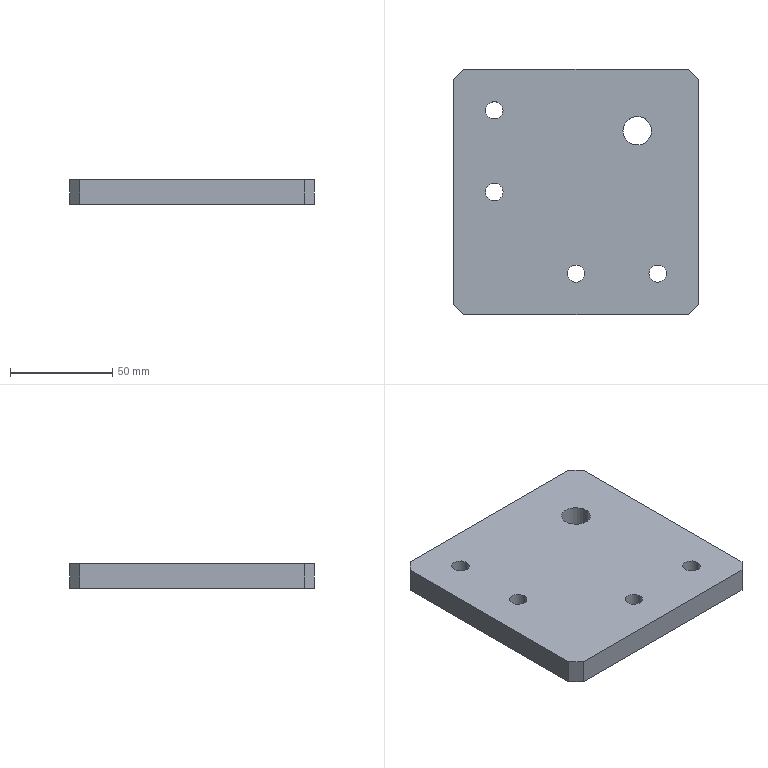Part | SolidWorks | features BaseBody 1 | 1 solid | 20 faces | box 120 x 120 x 12 mm | volume 167629 mm3 | cylinder 10 | plane 10 | commonest cylinder face diameters 8.5 x8 14 x2
STEP:
#1=CARTESIAN_POINT('',(37.,30.,-6.));
#2=VERTEX_POINT('',#1);
#3=CARTESIAN_POINT('',(23.,30.,-6.));
#4=VERTEX_POINT('',#3);
#5=CARTESIAN_POINT('',(30.,30.,-6.));
#6=DIRECTION('',(0.,0.,-1.));
#7=DIRECTION('',(-1.,0.,0.));
#8=AXIS2_PLACEMENT_3D('',#5,#6,#7);
#9=CIRCLE('',#8,7.);
#10=EDGE_CURVE('',#2,#4,#9,.T.);
#11=ORIENTED_EDGE('',*,*,#10,.T.);
#12=CARTESIAN_POINT('',(23.,30.,6.));
#13=VERTEX_POINT('',#12);
#14=CARTESIAN_POINT('',(23.,30.,6.));
#15=DIRECTION('',(0.,0.,1.));
#16=VECTOR('',#15,1000.);
#17=LINE('',#14,#16);
#18=EDGE_CURVE('',#4,#13,#17,.T.);
#19=ORIENTED_EDGE('',*,*,#18,.T.);
#20=CARTESIAN_POINT('',(37.,30.,6.));
#21=VERTEX_POINT('',#20);
#22=CARTESIAN_POINT('',(30.,30.,6.));
#23=DIRECTION('',(0.,0.,1.));
#24=DIRECTION('',(1.,0.,0.));
#25=AXIS2_PLACEMENT_3D('',#22,#23,#24);
#26=CIRCLE('',#25,7.);
#27=EDGE_CURVE('',#13,#21,#26,.T.);
#28=ORIENTED_EDGE('',*,*,#27,.T.);
#29=CARTESIAN_POINT('',(37.,30.,6.));
#30=DIRECTION('',(0.,0.,1.));
#31=VECTOR('',#30,1000.);
#32=LINE('',#29,#31);
#33=EDGE_CURVE('',#2,#21,#32,.T.);
#34=ORIENTED_EDGE('',*,*,#33,.F.);
#35=EDGE_LOOP('',(#11,#19,#28,#34));
#36=FACE_OUTER_BOUND('',#35,.T.);
#37=CARTESIAN_POINT('',(30.,30.,6.));
#38=DIRECTION('',(0.,0.,1.));
#39=DIRECTION('',(1.,0.,0.));
#40=AXIS2_PLACEMENT_3D('',#37,#38,#39);
#41=CYLINDRICAL_SURFACE('',#40,7.);
#42=ADVANCED_FACE('',(#36),#41,.F.);
#43=CARTESIAN_POINT('',(-4.25,-40.,-6.));
#44=VERTEX_POINT('',#43);
#45=CARTESIAN_POINT('',(4.25,-40.,-6.));
#46=VERTEX_POINT('',#45);
#47=CARTESIAN_POINT('',(0.,-40.,-6.));
#48=DIRECTION('',(0.,0.,1.));
#49=DIRECTION('',(1.,0.,0.));
#50=AXIS2_PLACEMENT_3D('',#47,#48,#49);
#51=CIRCLE('',#50,4.25);
#52=EDGE_CURVE('',#44,#46,#51,.T.);
#53=ORIENTED_EDGE('',*,*,#52,.F.);
#54=CARTESIAN_POINT('',(-4.25,-40.,6.));
#55=VERTEX_POINT('',#54);
#56=CARTESIAN_POINT('',(-4.25,-40.,-6.));
#57=DIRECTION('',(0.,0.,1.));
#58=VECTOR('',#57,1000.);
#59=LINE('',#56,#58);
#60=EDGE_CURVE('',#44,#55,#59,.T.);
#61=ORIENTED_EDGE('',*,*,#60,.T.);
#62=CARTESIAN_POINT('',(4.25,-40.,6.));
#63=VERTEX_POINT('',#62);
#64=CARTESIAN_POINT('',(0.,-40.,6.));
#65=DIRECTION('',(0.,0.,1.));
#66=DIRECTION('',(1.,0.,0.));
#67=AXIS2_PLACEMENT_3D('',#64,#65,#66);
#68=CIRCLE('',#67,4.25);
#69=EDGE_CURVE('',#55,#63,#68,.T.);
#70=ORIENTED_EDGE('',*,*,#69,.T.);
#71=CARTESIAN_POINT('',(4.25,-40.,-6.));
#72=DIRECTION('',(0.,0.,1.));
#73=VECTOR('',#72,1000.);
#74=LINE('',#71,#73);
#75=EDGE_CURVE('',#46,#63,#74,.T.);
#76=ORIENTED_EDGE('',*,*,#75,.F.);
#77=EDGE_LOOP('',(#53,#61,#70,#76));
#78=FACE_OUTER_BOUND('',#77,.T.);
#79=CARTESIAN_POINT('',(0.,-40.,-6.));
#80=DIRECTION('',(0.,0.,1.));
#81=DIRECTION('',(1.,0.,0.));
#82=AXIS2_PLACEMENT_3D('',#79,#80,#81);
#83=CYLINDRICAL_SURFACE('',#82,4.25);
#84=ADVANCED_FACE('',(#78),#83,.F.);
#85=CARTESIAN_POINT('',(35.75,-40.,-6.));
#86=VERTEX_POINT('',#85);
#87=CARTESIAN_POINT('',(44.25,-40.,-6.));
#88=VERTEX_POINT('',#87);
#89=CARTESIAN_POINT('',(40.,-40.,-6.));
#90=DIRECTION('',(0.,0.,1.));
#91=DIRECTION('',(1.,0.,0.));
#92=AXIS2_PLACEMENT_3D('',#89,#90,#91);
#93=CIRCLE('',#92,4.25);
#94=EDGE_CURVE('',#86,#88,#93,.T.);
#95=ORIENTED_EDGE('',*,*,#94,.F.);
#96=CARTESIAN_POINT('',(35.75,-40.,6.));
#97=VERTEX_POINT('',#96);
#98=CARTESIAN_POINT('',(35.75,-40.,-6.));
#99=DIRECTION('',(0.,0.,1.));
#100=VECTOR('',#99,1000.);
#101=LINE('',#98,#100);
#102=EDGE_CURVE('',#86,#97,#101,.T.);
#103=ORIENTED_EDGE('',*,*,#102,.T.);
#104=CARTESIAN_POINT('',(44.25,-40.,6.));
#105=VERTEX_POINT('',#104);
#106=CARTESIAN_POINT('',(40.,-40.,6.));
#107=DIRECTION('',(0.,0.,1.));
#108=DIRECTION('',(1.,0.,0.));
#109=AXIS2_PLACEMENT_3D('',#106,#107,#108);
#110=CIRCLE('',#109,4.25);
#111=EDGE_CURVE('',#97,#105,#110,.T.);
#112=ORIENTED_EDGE('',*,*,#111,.T.);
#113=CARTESIAN_POINT('',(44.25,-40.,-6.));
#114=DIRECTION('',(0.,0.,1.));
#115=VECTOR('',#114,1000.);
#116=LINE('',#113,#115);
#117=EDGE_CURVE('',#88,#105,#116,.T.);
#118=ORIENTED_EDGE('',*,*,#117,.F.);
#119=EDGE_LOOP('',(#95,#103,#112,#118));
#120=FACE_OUTER_BOUND('',#119,.T.);
#121=CARTESIAN_POINT('',(40.,-40.,-6.));
#122=DIRECTION('',(0.,0.,1.));
#123=DIRECTION('',(1.,0.,0.));
#124=AXIS2_PLACEMENT_3D('',#121,#122,#123);
#125=CYLINDRICAL_SURFACE('',#124,4.25);
#126=ADVANCED_FACE('',(#120),#125,.F.);
#127=CARTESIAN_POINT('',(-44.25,0.,-6.));
#128=VERTEX_POINT('',#127);
#129=CARTESIAN_POINT('',(-35.75,0.,-6.));
#130=VERTEX_POINT('',#129);
#131=CARTESIAN_POINT('',(-40.,0.,-6.));
#132=DIRECTION('',(0.,0.,1.));
#133=DIRECTION('',(1.,0.,0.));
#134=AXIS2_PLACEMENT_3D('',#131,#132,#133);
#135=CIRCLE('',#134,4.25);
#136=EDGE_CURVE('',#128,#130,#135,.T.);
#137=ORIENTED_EDGE('',*,*,#136,.F.);
#138=CARTESIAN_POINT('',(-44.25,0.,6.));
#139=VERTEX_POINT('',#138);
#140=CARTESIAN_POINT('',(-44.25,0.,-6.));
#141=DIRECTION('',(0.,0.,1.));
#142=VECTOR('',#141,1000.);
#143=LINE('',#140,#142);
#144=EDGE_CURVE('',#128,#139,#143,.T.);
#145=ORIENTED_EDGE('',*,*,#144,.T.);
#146=CARTESIAN_POINT('',(-35.75,0.,6.));
#147=VERTEX_POINT('',#146);
#148=CARTESIAN_POINT('',(-40.,0.,6.));
#149=DIRECTION('',(0.,0.,1.));
#150=DIRECTION('',(1.,0.,0.));
#151=AXIS2_PLACEMENT_3D('',#148,#149,#150);
#152=CIRCLE('',#151,4.25);
#153=EDGE_CURVE('',#139,#147,#152,.T.);
#154=ORIENTED_EDGE('',*,*,#153,.T.);
#155=CARTESIAN_POINT('',(-35.75,0.,-6.));
#156=DIRECTION('',(0.,0.,1.));
#157=VECTOR('',#156,1000.);
#158=LINE('',#155,#157);
#159=EDGE_CURVE('',#130,#147,#158,.T.);
#160=ORIENTED_EDGE('',*,*,#159,.F.);
#161=EDGE_LOOP('',(#137,#145,#154,#160));
#162=FACE_OUTER_BOUND('',#161,.T.);
#163=CARTESIAN_POINT('',(-40.,0.,-6.));
#164=DIRECTION('',(0.,0.,1.));
#165=DIRECTION('',(1.,0.,0.));
#166=AXIS2_PLACEMENT_3D('',#163,#164,#165);
#167=CYLINDRICAL_SURFACE('',#166,4.25);
#168=ADVANCED_FACE('',(#162),#167,.F.);
#169=CARTESIAN_POINT('',(-44.25,40.,-6.));
#170=VERTEX_POINT('',#169);
#171=CARTESIAN_POINT('',(-35.75,40.,-6.));
#172=VERTEX_POINT('',#171);
#173=CARTESIAN_POINT('',(-40.,40.,-6.));
#174=DIRECTION('',(0.,0.,1.));
#175=DIRECTION('',(1.,0.,0.));
#176=AXIS2_PLACEMENT_3D('',#173,#174,#175);
#177=CIRCLE('',#176,4.25);
#178=EDGE_CURVE('',#170,#172,#177,.T.);
#179=ORIENTED_EDGE('',*,*,#178,.F.);
#180=CARTESIAN_POINT('',(-44.25,40.,6.));
#181=VERTEX_POINT('',#180);
#182=CARTESIAN_POINT('',(-44.25,40.,-6.));
#183=DIRECTION('',(0.,0.,1.));
#184=VECTOR('',#183,1000.);
#185=LINE('',#182,#184);
#186=EDGE_CURVE('',#170,#181,#185,.T.);
#187=ORIENTED_EDGE('',*,*,#186,.T.);
#188=CARTESIAN_POINT('',(-35.75,40.,6.));
#189=VERTEX_POINT('',#188);
#190=CARTESIAN_POINT('',(-40.,40.,6.));
#191=DIRECTION('',(0.,0.,1.));
#192=DIRECTION('',(1.,0.,0.));
#193=AXIS2_PLACEMENT_3D('',#190,#191,#192);
#194=CIRCLE('',#193,4.25);
#195=EDGE_CURVE('',#181,#189,#194,.T.);
#196=ORIENTED_EDGE('',*,*,#195,.T.);
#197=CARTESIAN_POINT('',(-35.75,40.,-6.));
#198=DIRECTION('',(0.,0.,1.));
#199=VECTOR('',#198,1000.);
#200=LINE('',#197,#199);
#201=EDGE_CURVE('',#172,#189,#200,.T.);
#202=ORIENTED_EDGE('',*,*,#201,.F.);
#203=EDGE_LOOP('',(#179,#187,#196,#202));
#204=FACE_OUTER_BOUND('',#203,.T.);
#205=CARTESIAN_POINT('',(-40.,40.,-6.));
#206=DIRECTION('',(0.,0.,1.));
#207=DIRECTION('',(1.,0.,0.));
#208=AXIS2_PLACEMENT_3D('',#205,#206,#207);
#209=CYLINDRICAL_SURFACE('',#208,4.25);
#210=ADVANCED_FACE('',(#204),#209,.F.);
#211=CARTESIAN_POINT('',(-60.,55.,6.));
#212=VERTEX_POINT('',#211);
#213=CARTESIAN_POINT('',(-60.,-55.,6.));
#214=VERTEX_POINT('',#213);
#215=CARTESIAN_POINT('',(-60.,60.,6.));
#216=DIRECTION('',(0.,-1.,0.));
#217=VECTOR('',#216,1000.);
#218=LINE('',#215,#217);
#219=EDGE_CURVE('',#212,#214,#218,.T.);
#220=ORIENTED_EDGE('',*,*,#219,.F.);
#221=CARTESIAN_POINT('',(-60.,55.,-6.));
#222=VERTEX_POINT('',#221);
#223=CARTESIAN_POINT('',(-60.,55.,6.));
#224=DIRECTION('',(0.,0.,-1.));
#225=VECTOR('',#224,1000.);
#226=LINE('',#223,#225);
#227=EDGE_CURVE('',#212,#222,#226,.T.);
#228=ORIENTED_EDGE('',*,*,#227,.T.);
#229=CARTESIAN_POINT('',(-60.,-55.,-6.));
#230=VERTEX_POINT('',#229);
#231=CARTESIAN_POINT('',(-60.,60.,-6.));
#232=DIRECTION('',(0.,-1.,0.));
#233=VECTOR('',#232,1000.);
#234=LINE('',#231,#233);
#235=EDGE_CURVE('',#222,#230,#234,.T.);
#236=ORIENTED_EDGE('',*,*,#235,.T.);
#237=CARTESIAN_POINT('',(-60.,-55.,6.));
#238=DIRECTION('',(0.,0.,1.));
#239=VECTOR('',#238,1000.);
#240=LINE('',#237,#239);
#241=EDGE_CURVE('',#230,#214,#240,.T.);
#242=ORIENTED_EDGE('',*,*,#241,.T.);
#243=EDGE_LOOP('',(#220,#228,#236,#242));
#244=FACE_OUTER_BOUND('',#243,.T.);
#245=CARTESIAN_POINT('',(-60.,60.,6.));
#246=DIRECTION('',(1.,0.,0.));
#247=DIRECTION('',(0.,1.,0.));
#248=AXIS2_PLACEMENT_3D('',#245,#246,#247);
#249=PLANE('',#248);
#250=ADVANCED_FACE('',(#244),#249,.F.);
#251=CARTESIAN_POINT('',(-55.,-60.,-6.));
#252=VERTEX_POINT('',#251);
#253=CARTESIAN_POINT('',(55.,-60.,-6.));
#254=VERTEX_POINT('',#253);
#255=CARTESIAN_POINT('',(60.,-60.,-6.));
#256=DIRECTION('',(1.,0.,0.));
#257=VECTOR('',#256,1000.);
#258=LINE('',#255,#257);
#259=EDGE_CURVE('',#252,#254,#258,.T.);
#260=ORIENTED_EDGE('',*,*,#259,.T.);
#261=CARTESIAN_POINT('',(55.,-60.,6.));
#262=VERTEX_POINT('',#261);
#263=CARTESIAN_POINT('',(55.,-60.,6.));
#264=DIRECTION('',(0.,0.,1.));
#265=VECTOR('',#264,1000.);
#266=LINE('',#263,#265);
#267=EDGE_CURVE('',#254,#262,#266,.T.);
#268=ORIENTED_EDGE('',*,*,#267,.T.);
#269=CARTESIAN_POINT('',(-55.,-60.,6.));
#270=VERTEX_POINT('',#269);
#271=CARTESIAN_POINT('',(60.,-60.,6.));
#272=DIRECTION('',(1.,0.,0.));
#273=VECTOR('',#272,1000.);
#274=LINE('',#271,#273);
#275=EDGE_CURVE('',#270,#262,#274,.T.);
#276=ORIENTED_EDGE('',*,*,#275,.F.);
#277=CARTESIAN_POINT('',(-55.,-60.,6.));
#278=DIRECTION('',(0.,0.,-1.));
#279=VECTOR('',#278,1000.);
#280=LINE('',#277,#279);
#281=EDGE_CURVE('',#270,#252,#280,.T.);
#282=ORIENTED_EDGE('',*,*,#281,.T.);
#283=EDGE_LOOP('',(#260,#268,#276,#282));
#284=FACE_OUTER_BOUND('',#283,.T.);
#285=CARTESIAN_POINT('',(60.,-60.,6.));
#286=DIRECTION('',(0.,1.,0.));
#287=DIRECTION('',(-1.,0.,0.));
#288=AXIS2_PLACEMENT_3D('',#285,#286,#287);
#289=PLANE('',#288);
#290=ADVANCED_FACE('',(#284),#289,.F.);
#291=CARTESIAN_POINT('',(60.,-55.,-6.));
#292=VERTEX_POINT('',#291);
#293=CARTESIAN_POINT('',(60.,55.,-6.));
#294=VERTEX_POINT('',#293);
#295=CARTESIAN_POINT('',(60.,60.,-6.));
#296=DIRECTION('',(0.,1.,0.));
#297=VECTOR('',#296,1000.);
#298=LINE('',#295,#297);
#299=EDGE_CURVE('',#292,#294,#298,.T.);
#300=ORIENTED_EDGE('',*,*,#299,.T.);
#301=CARTESIAN_POINT('',(60.,55.,6.));
#302=VERTEX_POINT('',#301);
#303=CARTESIAN_POINT('',(60.,55.,6.));
#304=DIRECTION('',(0.,0.,1.));
#305=VECTOR('',#304,1000.);
#306=LINE('',#303,#305);
#307=EDGE_CURVE('',#294,#302,#306,.T.);
#308=ORIENTED_EDGE('',*,*,#307,.T.);
#309=CARTESIAN_POINT('',(60.,-55.,6.));
#310=VERTEX_POINT('',#309);
#311=CARTESIAN_POINT('',(60.,60.,6.));
#312=DIRECTION('',(0.,1.,0.));
#313=VECTOR('',#312,1000.);
#314=LINE('',#311,#313);
#315=EDGE_CURVE('',#310,#302,#314,.T.);
#316=ORIENTED_EDGE('',*,*,#315,.F.);
#317=CARTESIAN_POINT('',(60.,-55.,6.));
#318=DIRECTION('',(0.,0.,-1.));
#319=VECTOR('',#318,1000.);
#320=LINE('',#317,#319);
#321=EDGE_CURVE('',#310,#292,#320,.T.);
#322=ORIENTED_EDGE('',*,*,#321,.T.);
#323=EDGE_LOOP('',(#300,#308,#316,#322));
#324=FACE_OUTER_BOUND('',#323,.T.);
#325=CARTESIAN_POINT('',(60.,60.,6.));
#326=DIRECTION('',(-1.,0.,0.));
#327=DIRECTION('',(0.,-1.,0.));
#328=AXIS2_PLACEMENT_3D('',#325,#326,#327);
#329=PLANE('',#328);
#330=ADVANCED_FACE('',(#324),#329,.F.);
#331=CARTESIAN_POINT('',(55.,60.,6.));
#332=VERTEX_POINT('',#331);
#333=CARTESIAN_POINT('',(-55.,60.,6.));
#334=VERTEX_POINT('',#333);
#335=CARTESIAN_POINT('',(60.,60.,6.));
#336=DIRECTION('',(-1.,0.,0.));
#337=VECTOR('',#336,1000.);
#338=LINE('',#335,#337);
#339=EDGE_CURVE('',#332,#334,#338,.T.);
#340=ORIENTED_EDGE('',*,*,#339,.F.);
#341=CARTESIAN_POINT('',(55.,60.,-6.));
#342=VERTEX_POINT('',#341);
#343=CARTESIAN_POINT('',(55.,60.,6.));
#344=DIRECTION('',(0.,0.,-1.));
#345=VECTOR('',#344,1000.);
#346=LINE('',#343,#345);
#347=EDGE_CURVE('',#332,#342,#346,.T.);
#348=ORIENTED_EDGE('',*,*,#347,.T.);
#349=CARTESIAN_POINT('',(-55.,60.,-6.));
#350=VERTEX_POINT('',#349);
#351=CARTESIAN_POINT('',(60.,60.,-6.));
#352=DIRECTION('',(-1.,0.,0.));
#353=VECTOR('',#352,1000.);
#354=LINE('',#351,#353);
#355=EDGE_CURVE('',#342,#350,#354,.T.);
#356=ORIENTED_EDGE('',*,*,#355,.T.);
#357=CARTESIAN_POINT('',(-55.,60.,6.));
#358=DIRECTION('',(0.,0.,1.));
#359=VECTOR('',#358,1000.);
#360=LINE('',#357,#359);
#361=EDGE_CURVE('',#350,#334,#360,.T.);
#362=ORIENTED_EDGE('',*,*,#361,.T.);
#363=EDGE_LOOP('',(#340,#348,#356,#362));
#364=FACE_OUTER_BOUND('',#363,.T.);
#365=CARTESIAN_POINT('',(60.,60.,6.));
#366=DIRECTION('',(0.,-1.,0.));
#367=DIRECTION('',(1.,0.,0.));
#368=AXIS2_PLACEMENT_3D('',#365,#366,#367);
#369=PLANE('',#368);
#370=ADVANCED_FACE('',(#364),#369,.F.);
#371=CARTESIAN_POINT('',(30.,30.,6.));
#372=DIRECTION('',(0.,0.,1.));
#373=DIRECTION('',(1.,0.,0.));
#374=AXIS2_PLACEMENT_3D('',#371,#372,#373);
#375=CIRCLE('',#374,7.);
#376=EDGE_CURVE('',#21,#13,#375,.T.);
#377=ORIENTED_EDGE('',*,*,#376,.F.);
#378=ORIENTED_EDGE('',*,*,#27,.F.);
#379=EDGE_LOOP('',(#377,#378));
#380=FACE_BOUND('',#379,.T.);
#381=CARTESIAN_POINT('',(0.,-40.,6.));
#382=DIRECTION('',(0.,0.,1.));
#383=DIRECTION('',(1.,0.,0.));
#384=AXIS2_PLACEMENT_3D('',#381,#382,#383);
#385=CIRCLE('',#384,4.25);
#386=EDGE_CURVE('',#63,#55,#385,.T.);
#387=ORIENTED_EDGE('',*,*,#386,.F.);
#388=ORIENTED_EDGE('',*,*,#69,.F.);
#389=EDGE_LOOP('',(#387,#388));
#390=FACE_BOUND('',#389,.T.);
#391=CARTESIAN_POINT('',(40.,-40.,6.));
#392=DIRECTION('',(0.,0.,1.));
#393=DIRECTION('',(1.,0.,0.));
#394=AXIS2_PLACEMENT_3D('',#391,#392,#393);
#395=CIRCLE('',#394,4.25);
#396=EDGE_CURVE('',#105,#97,#395,.T.);
#397=ORIENTED_EDGE('',*,*,#396,.F.);
#398=ORIENTED_EDGE('',*,*,#111,.F.);
#399=EDGE_LOOP('',(#397,#398));
#400=FACE_BOUND('',#399,.T.);
#401=CARTESIAN_POINT('',(-40.,0.,6.));
#402=DIRECTION('',(0.,0.,1.));
#403=DIRECTION('',(1.,0.,0.));
#404=AXIS2_PLACEMENT_3D('',#401,#402,#403);
#405=CIRCLE('',#404,4.25);
#406=EDGE_CURVE('',#147,#139,#405,.T.);
#407=ORIENTED_EDGE('',*,*,#406,.F.);
#408=ORIENTED_EDGE('',*,*,#153,.F.);
#409=EDGE_LOOP('',(#407,#408));
#410=FACE_BOUND('',#409,.T.);
#411=CARTESIAN_POINT('',(-40.,40.,6.));
#412=DIRECTION('',(0.,0.,1.));
#413=DIRECTION('',(1.,0.,0.));
#414=AXIS2_PLACEMENT_3D('',#411,#412,#413);
#415=CIRCLE('',#414,4.25);
#416=EDGE_CURVE('',#189,#181,#415,.T.);
#417=ORIENTED_EDGE('',*,*,#416,.F.);
#418=ORIENTED_EDGE('',*,*,#195,.F.);
#419=EDGE_LOOP('',(#417,#418));
#420=FACE_BOUND('',#419,.T.);
#421=ORIENTED_EDGE('',*,*,#315,.T.);
#422=CARTESIAN_POINT('',(55.,60.,6.));
#423=DIRECTION('',(-0.7071,0.7071,0.));
#424=VECTOR('',#423,1000.);
#425=LINE('',#422,#424);
#426=EDGE_CURVE('',#302,#332,#425,.T.);
#427=ORIENTED_EDGE('',*,*,#426,.T.);
#428=ORIENTED_EDGE('',*,*,#339,.T.);
#429=CARTESIAN_POINT('',(-60.,55.,6.));
#430=DIRECTION('',(-0.7071,-0.7071,0.));
#431=VECTOR('',#430,1000.);
#432=LINE('',#429,#431);
#433=EDGE_CURVE('',#334,#212,#432,.T.);
#434=ORIENTED_EDGE('',*,*,#433,.T.);
#435=ORIENTED_EDGE('',*,*,#219,.T.);
#436=CARTESIAN_POINT('',(-55.,-60.,6.));
#437=DIRECTION('',(0.7071,-0.7071,0.));
#438=VECTOR('',#437,1000.);
#439=LINE('',#436,#438);
#440=EDGE_CURVE('',#214,#270,#439,.T.);
#441=ORIENTED_EDGE('',*,*,#440,.T.);
#442=ORIENTED_EDGE('',*,*,#275,.T.);
#443=CARTESIAN_POINT('',(60.,-55.,6.));
#444=DIRECTION('',(0.7071,0.7071,0.));
#445=VECTOR('',#444,1000.);
#446=LINE('',#443,#445);
#447=EDGE_CURVE('',#262,#310,#446,.T.);
#448=ORIENTED_EDGE('',*,*,#447,.T.);
#449=EDGE_LOOP('',(#421,#427,#428,#434,#435,#441,#442,#448));
#450=FACE_OUTER_BOUND('',#449,.T.);
#451=CARTESIAN_POINT('',(-60.,-60.,6.));
#452=DIRECTION('',(0.,0.,-1.));
#453=DIRECTION('',(-1.,0.,0.));
#454=AXIS2_PLACEMENT_3D('',#451,#452,#453);
#455=PLANE('',#454);
#456=ADVANCED_FACE('',(#380,#390,#400,#410,#420,#450),#455,.F.);
#457=ORIENTED_EDGE('',*,*,#10,.F.);
#458=CARTESIAN_POINT('',(30.,30.,-6.));
#459=DIRECTION('',(0.,0.,-1.));
#460=DIRECTION('',(-1.,0.,0.));
#461=AXIS2_PLACEMENT_3D('',#458,#459,#460);
#462=CIRCLE('',#461,7.);
#463=EDGE_CURVE('',#4,#2,#462,.T.);
#464=ORIENTED_EDGE('',*,*,#463,.F.);
#465=EDGE_LOOP('',(#457,#464));
#466=FACE_BOUND('',#465,.T.);
#467=CARTESIAN_POINT('',(0.,-40.,-6.));
#468=DIRECTION('',(0.,0.,1.));
#469=DIRECTION('',(1.,0.,0.));
#470=AXIS2_PLACEMENT_3D('',#467,#468,#469);
#471=CIRCLE('',#470,4.25);
#472=EDGE_CURVE('',#46,#44,#471,.T.);
#473=ORIENTED_EDGE('',*,*,#472,.T.);
#474=ORIENTED_EDGE('',*,*,#52,.T.);
#475=EDGE_LOOP('',(#473,#474));
#476=FACE_BOUND('',#475,.T.);
#477=CARTESIAN_POINT('',(40.,-40.,-6.));
#478=DIRECTION('',(0.,0.,1.));
#479=DIRECTION('',(1.,0.,0.));
#480=AXIS2_PLACEMENT_3D('',#477,#478,#479);
#481=CIRCLE('',#480,4.25);
#482=EDGE_CURVE('',#88,#86,#481,.T.);
#483=ORIENTED_EDGE('',*,*,#482,.T.);
#484=ORIENTED_EDGE('',*,*,#94,.T.);
#485=EDGE_LOOP('',(#483,#484));
#486=FACE_BOUND('',#485,.T.);
#487=CARTESIAN_POINT('',(-40.,0.,-6.));
#488=DIRECTION('',(0.,0.,1.));
#489=DIRECTION('',(1.,0.,0.));
#490=AXIS2_PLACEMENT_3D('',#487,#488,#489);
#491=CIRCLE('',#490,4.25);
#492=EDGE_CURVE('',#130,#128,#491,.T.);
#493=ORIENTED_EDGE('',*,*,#492,.T.);
#494=ORIENTED_EDGE('',*,*,#136,.T.);
#495=EDGE_LOOP('',(#493,#494));
#496=FACE_BOUND('',#495,.T.);
#497=CARTESIAN_POINT('',(-40.,40.,-6.));
#498=DIRECTION('',(0.,0.,1.));
#499=DIRECTION('',(1.,0.,0.));
#500=AXIS2_PLACEMENT_3D('',#497,#498,#499);
#501=CIRCLE('',#500,4.25);
#502=EDGE_CURVE('',#172,#170,#501,.T.);
#503=ORIENTED_EDGE('',*,*,#502,.T.);
#504=ORIENTED_EDGE('',*,*,#178,.T.);
#505=EDGE_LOOP('',(#503,#504));
#506=FACE_BOUND('',#505,.T.);
#507=ORIENTED_EDGE('',*,*,#355,.F.);
#508=CARTESIAN_POINT('',(57.5,57.5,-6.));
#509=DIRECTION('',(0.7071,-0.7071,0.));
#510=VECTOR('',#509,1000.);
#511=LINE('',#508,#510);
#512=EDGE_CURVE('',#342,#294,#511,.T.);
#513=ORIENTED_EDGE('',*,*,#512,.T.);
#514=ORIENTED_EDGE('',*,*,#299,.F.);
#515=CARTESIAN_POINT('',(-2.5,-117.5,-6.));
#516=DIRECTION('',(-0.7071,-0.7071,0.));
#517=VECTOR('',#516,1000.);
#518=LINE('',#515,#517);
#519=EDGE_CURVE('',#292,#254,#518,.T.);
#520=ORIENTED_EDGE('',*,*,#519,.T.);
#521=ORIENTED_EDGE('',*,*,#259,.F.);
#522=CARTESIAN_POINT('',(-57.5,-57.5,-6.));
#523=DIRECTION('',(-0.7071,0.7071,0.));
#524=VECTOR('',#523,1000.);
#525=LINE('',#522,#524);
#526=EDGE_CURVE('',#252,#230,#525,.T.);
#527=ORIENTED_EDGE('',*,*,#526,.T.);
#528=ORIENTED_EDGE('',*,*,#235,.F.);
#529=CARTESIAN_POINT('',(-117.5,-2.5,-6.));
#530=DIRECTION('',(0.7071,0.7071,0.));
#531=VECTOR('',#530,1000.);
#532=LINE('',#529,#531);
#533=EDGE_CURVE('',#222,#350,#532,.T.);
#534=ORIENTED_EDGE('',*,*,#533,.T.);
#535=EDGE_LOOP('',(#507,#513,#514,#520,#521,#527,#528,#534));
#536=FACE_OUTER_BOUND('',#535,.T.);
#537=CARTESIAN_POINT('',(-60.,-60.,-6.));
#538=DIRECTION('',(0.,0.,-1.));
#539=DIRECTION('',(-1.,0.,0.));
#540=AXIS2_PLACEMENT_3D('',#537,#538,#539);
#541=PLANE('',#540);
#542=ADVANCED_FACE('',(#466,#476,#486,#496,#506,#536),#541,.T.);
#543=ORIENTED_EDGE('',*,*,#186,.F.);
#544=ORIENTED_EDGE('',*,*,#502,.F.);
#545=ORIENTED_EDGE('',*,*,#201,.T.);
#546=ORIENTED_EDGE('',*,*,#416,.T.);
#547=EDGE_LOOP('',(#543,#544,#545,#546));
#548=FACE_OUTER_BOUND('',#547,.T.);
#549=CARTESIAN_POINT('',(-40.,40.,-6.));
#550=DIRECTION('',(0.,0.,1.));
#551=DIRECTION('',(1.,0.,0.));
#552=AXIS2_PLACEMENT_3D('',#549,#550,#551);
#553=CYLINDRICAL_SURFACE('',#552,4.25);
#554=ADVANCED_FACE('',(#548),#553,.F.);
#555=ORIENTED_EDGE('',*,*,#144,.F.);
#556=ORIENTED_EDGE('',*,*,#492,.F.);
#557=ORIENTED_EDGE('',*,*,#159,.T.);
#558=ORIENTED_EDGE('',*,*,#406,.T.);
#559=EDGE_LOOP('',(#555,#556,#557,#558));
#560=FACE_OUTER_BOUND('',#559,.T.);
#561=CARTESIAN_POINT('',(-40.,0.,-6.));
#562=DIRECTION('',(0.,0.,1.));
#563=DIRECTION('',(1.,0.,0.));
#564=AXIS2_PLACEMENT_3D('',#561,#562,#563);
#565=CYLINDRICAL_SURFACE('',#564,4.25);
#566=ADVANCED_FACE('',(#560),#565,.F.);
#567=ORIENTED_EDGE('',*,*,#102,.F.);
#568=ORIENTED_EDGE('',*,*,#482,.F.);
#569=ORIENTED_EDGE('',*,*,#117,.T.);
#570=ORIENTED_EDGE('',*,*,#396,.T.);
#571=EDGE_LOOP('',(#567,#568,#569,#570));
#572=FACE_OUTER_BOUND('',#571,.T.);
#573=CARTESIAN_POINT('',(40.,-40.,-6.));
#574=DIRECTION('',(0.,0.,1.));
#575=DIRECTION('',(1.,0.,0.));
#576=AXIS2_PLACEMENT_3D('',#573,#574,#575);
#577=CYLINDRICAL_SURFACE('',#576,4.25);
#578=ADVANCED_FACE('',(#572),#577,.F.);
#579=ORIENTED_EDGE('',*,*,#60,.F.);
#580=ORIENTED_EDGE('',*,*,#472,.F.);
#581=ORIENTED_EDGE('',*,*,#75,.T.);
#582=ORIENTED_EDGE('',*,*,#386,.T.);
#583=EDGE_LOOP('',(#579,#580,#581,#582));
#584=FACE_OUTER_BOUND('',#583,.T.);
#585=CARTESIAN_POINT('',(0.,-40.,-6.));
#586=DIRECTION('',(0.,0.,1.));
#587=DIRECTION('',(1.,0.,0.));
#588=AXIS2_PLACEMENT_3D('',#585,#586,#587);
#589=CYLINDRICAL_SURFACE('',#588,4.25);
#590=ADVANCED_FACE('',(#584),#589,.F.);
#591=ORIENTED_EDGE('',*,*,#18,.F.);
#592=ORIENTED_EDGE('',*,*,#463,.T.);
#593=ORIENTED_EDGE('',*,*,#33,.T.);
#594=ORIENTED_EDGE('',*,*,#376,.T.);
#595=EDGE_LOOP('',(#591,#592,#593,#594));
#596=FACE_OUTER_BOUND('',#595,.T.);
#597=CARTESIAN_POINT('',(30.,30.,6.));
#598=DIRECTION('',(0.,0.,1.));
#599=DIRECTION('',(1.,0.,0.));
#600=AXIS2_PLACEMENT_3D('',#597,#598,#599);
#601=CYLINDRICAL_SURFACE('',#600,7.);
#602=ADVANCED_FACE('',(#596),#601,.F.);
#603=ORIENTED_EDGE('',*,*,#426,.F.);
#604=ORIENTED_EDGE('',*,*,#307,.F.);
#605=ORIENTED_EDGE('',*,*,#512,.F.);
#606=ORIENTED_EDGE('',*,*,#347,.F.);
#607=EDGE_LOOP('',(#603,#604,#605,#606));
#608=FACE_OUTER_BOUND('',#607,.T.);
#609=CARTESIAN_POINT('',(55.,60.,6.));
#610=DIRECTION('',(-0.7071,-0.7071,0.));
#611=DIRECTION('',(0.7071,-0.7071,0.));
#612=AXIS2_PLACEMENT_3D('',#609,#610,#611);
#613=PLANE('',#612);
#614=ADVANCED_FACE('',(#608),#613,.F.);
#615=ORIENTED_EDGE('',*,*,#447,.F.);
#616=ORIENTED_EDGE('',*,*,#267,.F.);
#617=ORIENTED_EDGE('',*,*,#519,.F.);
#618=ORIENTED_EDGE('',*,*,#321,.F.);
#619=EDGE_LOOP('',(#615,#616,#617,#618));
#620=FACE_OUTER_BOUND('',#619,.T.);
#621=CARTESIAN_POINT('',(60.,-55.,6.));
#622=DIRECTION('',(-0.7071,0.7071,0.));
#623=DIRECTION('',(-0.7071,-0.7071,0.));
#624=AXIS2_PLACEMENT_3D('',#621,#622,#623);
#625=PLANE('',#624);
#626=ADVANCED_FACE('',(#620),#625,.F.);
#627=ORIENTED_EDGE('',*,*,#433,.F.);
#628=ORIENTED_EDGE('',*,*,#361,.F.);
#629=ORIENTED_EDGE('',*,*,#533,.F.);
#630=ORIENTED_EDGE('',*,*,#227,.F.);
#631=EDGE_LOOP('',(#627,#628,#629,#630));
#632=FACE_OUTER_BOUND('',#631,.T.);
#633=CARTESIAN_POINT('',(-60.,55.,6.));
#634=DIRECTION('',(0.7071,-0.7071,0.));
#635=DIRECTION('',(0.7071,0.7071,0.));
#636=AXIS2_PLACEMENT_3D('',#633,#634,#635);
#637=PLANE('',#636);
#638=ADVANCED_FACE('',(#632),#637,.F.);
#639=ORIENTED_EDGE('',*,*,#440,.F.);
#640=ORIENTED_EDGE('',*,*,#241,.F.);
#641=ORIENTED_EDGE('',*,*,#526,.F.);
#642=ORIENTED_EDGE('',*,*,#281,.F.);
#643=EDGE_LOOP('',(#639,#640,#641,#642));
#644=FACE_OUTER_BOUND('',#643,.T.);
#645=CARTESIAN_POINT('',(-55.,-60.,6.));
#646=DIRECTION('',(0.7071,0.7071,0.));
#647=DIRECTION('',(-0.7071,0.7071,0.));
#648=AXIS2_PLACEMENT_3D('',#645,#646,#647);
#649=PLANE('',#648);
#650=ADVANCED_FACE('',(#644),#649,.F.);
#651=CLOSED_SHELL('',(#42,#84,#126,#168,#210,#250,#290,#330,#370,#456,#542,#554,#566,#578,#590,#602,#614,#626,#638,#650));
#652=MANIFOLD_SOLID_BREP('',#651);
#653=CARTESIAN_POINT('',(0.,0.,0.));
#654=DIRECTION('',(0.,0.,1.));
#655=DIRECTION('',(1.,0.,0.));
#656=AXIS2_PLACEMENT_3D('',#653,#654,#655);
#657=(LENGTH_UNIT()NAMED_UNIT(*)SI_UNIT(.MILLI.,.METRE.));
#658=UNCERTAINTY_MEASURE_WITH_UNIT(LENGTH_MEASURE(0.00001),#657,'','');
#659=(NAMED_UNIT(*)PLANE_ANGLE_UNIT()SI_UNIT($,.RADIAN.));
#660=(NAMED_UNIT(*)SI_UNIT($,.STERADIAN.)SOLID_ANGLE_UNIT());
#661=(GEOMETRIC_REPRESENTATION_CONTEXT(3)GLOBAL_UNCERTAINTY_ASSIGNED_CONTEXT((#658))GLOBAL_UNIT_ASSIGNED_CONTEXT((#657,#659,#660))REPRESENTATION_CONTEXT('',''));
#662=ADVANCED_BREP_SHAPE_REPRESENTATION('',(#652,#656),#661);